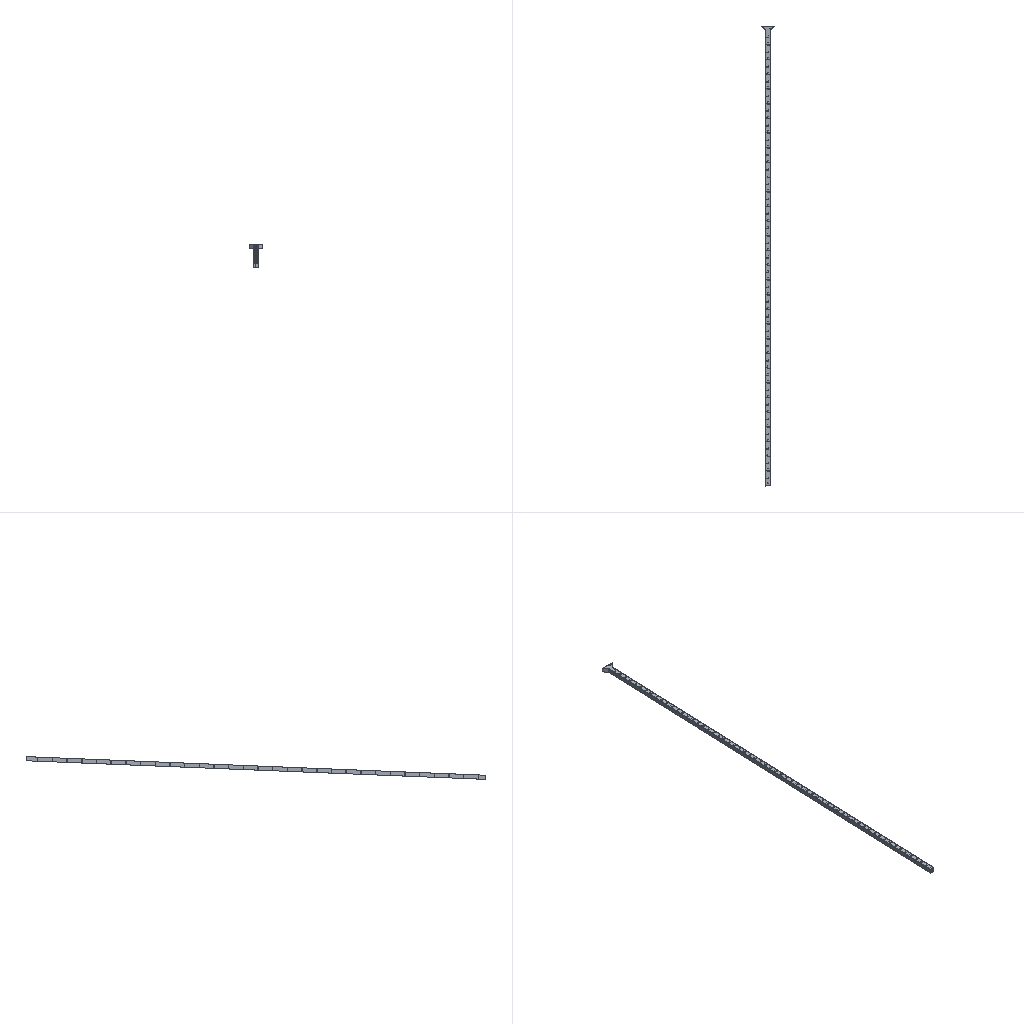Simulation study | ansys fluent
Set-up summary:
category,name,step,type,value,unit,region
solver,ansys_fluent,,Fluent 26.1.0
units,SI m-kg-s (Fluent internal),,stated,boundary values in the units shown in brackets; results in listed units
analysis,deck.cas,,cfd steady,"dimension=3D; solver=3d, dp, pbns, vof, rngke (3d, double precision, pressure-based, VOF, RNG k-epsilon); source_case=.cas"
model,Space,deck.cas,,3D
model,Time,deck.cas,,Steady
model,Viscous,deck.cas,,RNG k-epsilon turbulence model
model,Wall Treatment,deck.cas,,Standard Wall Functions
model,Heat Transfer,deck.cas,,Disabled
model,Multiphase,deck.cas,,Volume of Fluid
mesh,nodes,,,809457
mesh,elements,,,718434
mesh,faces,,,2243617
cell_zone,part_1 (mixture),deck.cas,fluid,material=water-liquid,,zone 3
cell_zone,part_1 (air),deck.cas,fluid,material=air,,zone 3
cell_zone,part_1 (water),deck.cas,fluid,material=water-liquid,,zone 3
material,water-liquid (fluid),,Density,998.2,kg/m^3
material,water-liquid (fluid),,Viscosity,0.001003,kg/(m s)
material,air (fluid),,Density,1.225,kg/m^3
material,air (fluid),,Viscosity,1.7894e-05,kg/(m s)
material,aluminum (solid),,Density,2719,kg/m^3
bc,out2 (mixture),deck.cas,pressure-outlet,Backflow Direction Specification Method=Normal to Boundary,,zone 11
bc,out2 (air),deck.cas,pressure-outlet,,,zone 11
bc,out2 (water),deck.cas,pressure-outlet,,,zone 11
bc,out1 (mixture),deck.cas,pressure-outlet,Backflow Direction Specification Method=Normal to Boundary,,zone 7
bc,out1 (air),deck.cas,pressure-outlet,,,zone 7
bc,out1 (water),deck.cas,pressure-outlet,,,zone 7
bc,int (mixture),deck.cas,velocity-inlet,Velocity Magnitude [m/s]=1,,zone 6
bc,int (air),deck.cas,velocity-inlet,,,zone 6
bc,int (water),deck.cas,velocity-inlet,Volume Fraction=1,,zone 6
bc,wall-part_1 (mixture),deck.cas,wall,Wall Motion=Stationary Wall; Shear Boundary Condition=No Slip,,zone 1
bc,wall-part_1 (air),deck.cas,wall,,,zone 1
bc,wall-part_1 (water),deck.cas,wall,,,zone 1
bc,wall1 (mixture),deck.cas,wall,Wall Motion=Stationary Wall; Shear Boundary Condition=No Slip,,zone 8
bc,wall1 (air),deck.cas,wall,,,zone 8
bc,wall1 (water),deck.cas,wall,,,zone 8
bc,wall2 (mixture),deck.cas,wall,Wall Motion=Stationary Wall; Shear Boundary Condition=No Slip,,zone 9
bc,wall2 (air),deck.cas,wall,,,zone 9
bc,wall2 (water),deck.cas,wall,,,zone 9
bc,wall3 (mixture),deck.cas,wall,Wall Motion=Stationary Wall; Shear Boundary Condition=No Slip,,zone 10
bc,wall3 (air),deck.cas,wall,,,zone 10
bc,wall3 (water),deck.cas,wall,,,zone 10
Results summary:
result,mass flow rate int,deck.cas,,107.806,kg/s
result,mass flow rate out1,deck.cas,,-106.102,kg/s
result,mass flow rate out2,deck.cas,,-0.5971,kg/s
result,mass flow rate wall-part_1,deck.cas,,-0,kg/s
result,mass flow rate wall1,deck.cas,,-0,kg/s
result,mass flow rate wall2,deck.cas,,-0,kg/s
result,mass flow rate wall3,deck.cas,,-0,kg/s
result,mass flow rate Net,deck.cas,,1.107,kg/s
result,wall force total wall-part_1,deck.cas,,"(-3.325, -157.669, 0.1819)",N
result,wall force pressure wall-part_1,deck.cas,,"(-3.245, -157.529, 0)",N
result,wall force viscous wall-part_1,deck.cas,,"(-0.08064, -0.1404, 0.1819)",N
result,wall force total wall1,deck.cas,,"(687.657, -72.788, 0.2318)",N
result,wall force pressure wall1,deck.cas,,"(687.995, -71.31, 0)",N
result,wall force viscous wall1,deck.cas,,"(-0.338, -1.478, 0.2318)",N
result,wall force total wall2,deck.cas,,"(-0.05017, 103.037, -2594.05)",N
result,wall force pressure wall2,deck.cas,,"(-0.0026, 105.091, -2593.97)",N
result,wall force viscous wall2,deck.cas,,"(-0.04757, -2.055, -0.08324)",N
result,wall force total wall3,deck.cas,,"(-686.439, -71.54, 0.2155)",N
result,wall force pressure wall3,deck.cas,,"(-686.754, -70.553, 0)",N
result,wall force viscous wall3,deck.cas,,"(0.3154, -0.9866, 0.2155)",N
result,wall force total Net,deck.cas,,"(-2.158, -198.96, -2593.42)",N
result,wall force pressure Net,deck.cas,,"(-2.007, -194.3, -2593.97)",N
result,wall force viscous Net,deck.cas,,"(-0.1509, -4.66, 0.5459)",N